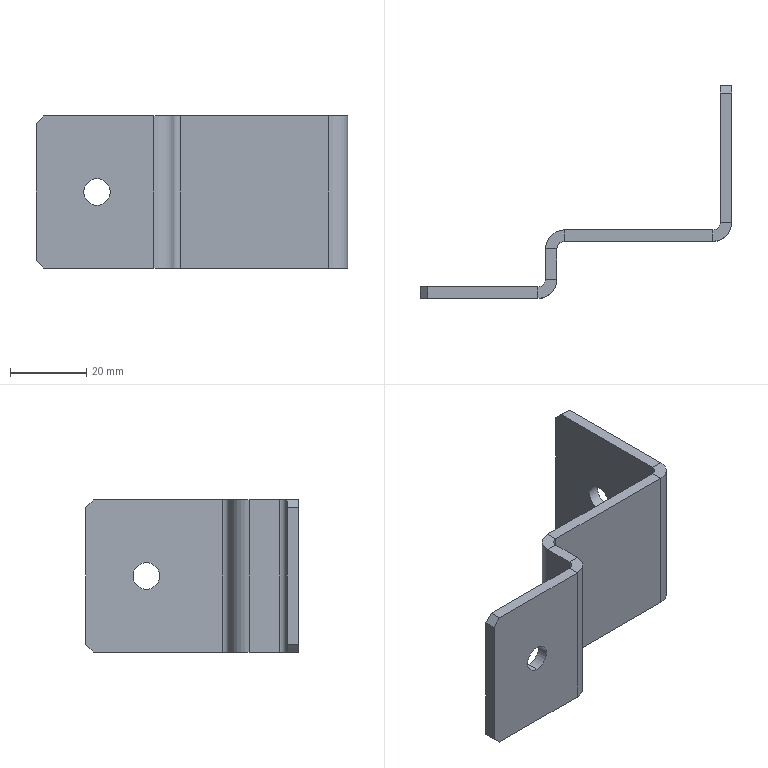Part | NX | features BREP 1 | 1 solid | 38 faces | box 82 x 56 x 40 mm | volume 15404 mm3 | plane 28 | cylinder 10 | commonest cylinder face diameters 7 x4 4 x3 10 x3
STEP:
#1=CARTESIAN_POINT('',(-34.,0.,20.));
#2=VERTEX_POINT('',#1);
#3=CARTESIAN_POINT('',(-36.,0.,18.));
#4=VERTEX_POINT('',#3);
#5=CARTESIAN_POINT('',(-36.,0.,18.));
#6=DIRECTION('',(-0.7071,0.,-0.7071));
#7=VECTOR('',#6,1000.);
#8=LINE('',#5,#7);
#9=EDGE_CURVE('',#2,#4,#8,.T.);
#10=ORIENTED_EDGE('',*,*,#9,.F.);
#11=CARTESIAN_POINT('',(-34.,3.,20.));
#12=VERTEX_POINT('',#11);
#13=CARTESIAN_POINT('',(-34.,5.,20.));
#14=DIRECTION('',(0.,-1.,0.));
#15=VECTOR('',#14,1000.);
#16=LINE('',#13,#15);
#17=EDGE_CURVE('',#12,#2,#16,.T.);
#18=ORIENTED_EDGE('',*,*,#17,.F.);
#19=CARTESIAN_POINT('',(-36.,3.,18.));
#20=VERTEX_POINT('',#19);
#21=CARTESIAN_POINT('',(-35.,3.,19.));
#22=DIRECTION('',(0.7071,0.,0.7071));
#23=VECTOR('',#22,1000.);
#24=LINE('',#21,#23);
#25=EDGE_CURVE('',#20,#12,#24,.T.);
#26=ORIENTED_EDGE('',*,*,#25,.F.);
#27=CARTESIAN_POINT('',(-36.,0.,18.));
#28=DIRECTION('',(0.,1.,0.));
#29=VECTOR('',#28,1000.);
#30=LINE('',#27,#29);
#31=EDGE_CURVE('',#4,#20,#30,.T.);
#32=ORIENTED_EDGE('',*,*,#31,.F.);
#33=EDGE_LOOP('',(#10,#18,#26,#32));
#34=FACE_BOUND('',#33,.T.);
#35=CARTESIAN_POINT('',(-36.,0.,18.));
#36=DIRECTION('',(0.7071,0.,-0.7071));
#37=DIRECTION('',(0.,1.,0.));
#38=AXIS2_PLACEMENT_3D('',#35,#36,#37);
#39=PLANE('',#38);
#40=ADVANCED_FACE('',(#34),#39,.F.);
#41=CARTESIAN_POINT('',(-36.,0.,-18.));
#42=VERTEX_POINT('',#41);
#43=CARTESIAN_POINT('',(-34.,0.,-20.));
#44=VERTEX_POINT('',#43);
#45=CARTESIAN_POINT('',(-34.,0.,-20.));
#46=DIRECTION('',(0.7071,0.,-0.7071));
#47=VECTOR('',#46,1000.);
#48=LINE('',#45,#47);
#49=EDGE_CURVE('',#42,#44,#48,.T.);
#50=ORIENTED_EDGE('',*,*,#49,.F.);
#51=CARTESIAN_POINT('',(-36.,3.,-18.));
#52=VERTEX_POINT('',#51);
#53=CARTESIAN_POINT('',(-36.,0.,-18.));
#54=DIRECTION('',(0.,-1.,0.));
#55=VECTOR('',#54,1000.);
#56=LINE('',#53,#55);
#57=EDGE_CURVE('',#52,#42,#56,.T.);
#58=ORIENTED_EDGE('',*,*,#57,.F.);
#59=CARTESIAN_POINT('',(-34.,3.,-20.));
#60=VERTEX_POINT('',#59);
#61=CARTESIAN_POINT('',(-55.,3.,1.));
#62=DIRECTION('',(-0.7071,0.,0.7071));
#63=VECTOR('',#62,1000.);
#64=LINE('',#61,#63);
#65=EDGE_CURVE('',#60,#52,#64,.T.);
#66=ORIENTED_EDGE('',*,*,#65,.F.);
#67=CARTESIAN_POINT('',(-34.,3.,-20.));
#68=DIRECTION('',(0.,1.,0.));
#69=VECTOR('',#68,1000.);
#70=LINE('',#67,#69);
#71=EDGE_CURVE('',#44,#60,#70,.T.);
#72=ORIENTED_EDGE('',*,*,#71,.F.);
#73=EDGE_LOOP('',(#50,#58,#66,#72));
#74=FACE_BOUND('',#73,.T.);
#75=CARTESIAN_POINT('',(-34.,20.,-20.));
#76=DIRECTION('',(-0.7071,0.,-0.7071));
#77=DIRECTION('',(0.,-1.,0.));
#78=AXIS2_PLACEMENT_3D('',#75,#76,#77);
#79=PLANE('',#78);
#80=ADVANCED_FACE('',(#74),#79,.T.);
#81=CARTESIAN_POINT('',(43.,54.,20.));
#82=VERTEX_POINT('',#81);
#83=CARTESIAN_POINT('',(43.,56.,18.));
#84=VERTEX_POINT('',#83);
#85=CARTESIAN_POINT('',(43.,34.5,39.5));
#86=DIRECTION('',(0.,0.7071,-0.7071));
#87=VECTOR('',#86,1000.);
#88=LINE('',#85,#87);
#89=EDGE_CURVE('',#82,#84,#88,.T.);
#90=ORIENTED_EDGE('',*,*,#89,.F.);
#91=CARTESIAN_POINT('',(46.,54.,20.));
#92=VERTEX_POINT('',#91);
#93=CARTESIAN_POINT('',(41.,54.,20.));
#94=DIRECTION('',(-1.,0.,0.));
#95=VECTOR('',#94,1000.);
#96=LINE('',#93,#95);
#97=EDGE_CURVE('',#92,#82,#96,.T.);
#98=ORIENTED_EDGE('',*,*,#97,.F.);
#99=CARTESIAN_POINT('',(46.,56.,18.));
#100=VERTEX_POINT('',#99);
#101=CARTESIAN_POINT('',(46.,56.,18.));
#102=DIRECTION('',(0.,-0.7071,0.7071));
#103=VECTOR('',#102,1000.);
#104=LINE('',#101,#103);
#105=EDGE_CURVE('',#100,#92,#104,.T.);
#106=ORIENTED_EDGE('',*,*,#105,.F.);
#107=CARTESIAN_POINT('',(43.,56.,18.));
#108=DIRECTION('',(1.,0.,0.));
#109=VECTOR('',#108,1000.);
#110=LINE('',#107,#109);
#111=EDGE_CURVE('',#84,#100,#110,.T.);
#112=ORIENTED_EDGE('',*,*,#111,.F.);
#113=EDGE_LOOP('',(#90,#98,#106,#112));
#114=FACE_BOUND('',#113,.T.);
#115=CARTESIAN_POINT('',(43.,56.,18.));
#116=DIRECTION('',(0.,-0.7071,-0.7071));
#117=DIRECTION('',(1.,0.,0.));
#118=AXIS2_PLACEMENT_3D('',#115,#116,#117);
#119=PLANE('',#118);
#120=ADVANCED_FACE('',(#114),#119,.F.);
#121=CARTESIAN_POINT('',(43.,56.,-18.));
#122=VERTEX_POINT('',#121);
#123=CARTESIAN_POINT('',(43.,54.,-20.));
#124=VERTEX_POINT('',#123);
#125=CARTESIAN_POINT('',(43.,54.5,-19.5));
#126=DIRECTION('',(0.,-0.7071,-0.7071));
#127=VECTOR('',#126,1000.);
#128=LINE('',#125,#127);
#129=EDGE_CURVE('',#122,#124,#128,.T.);
#130=ORIENTED_EDGE('',*,*,#129,.F.);
#131=CARTESIAN_POINT('',(46.,56.,-18.));
#132=VERTEX_POINT('',#131);
#133=CARTESIAN_POINT('',(43.,56.,-18.));
#134=DIRECTION('',(-1.,0.,0.));
#135=VECTOR('',#134,1000.);
#136=LINE('',#133,#135);
#137=EDGE_CURVE('',#132,#122,#136,.T.);
#138=ORIENTED_EDGE('',*,*,#137,.F.);
#139=CARTESIAN_POINT('',(46.,54.,-20.));
#140=VERTEX_POINT('',#139);
#141=CARTESIAN_POINT('',(46.,54.,-20.));
#142=DIRECTION('',(0.,0.7071,0.7071));
#143=VECTOR('',#142,1000.);
#144=LINE('',#141,#143);
#145=EDGE_CURVE('',#140,#132,#144,.T.);
#146=ORIENTED_EDGE('',*,*,#145,.F.);
#147=CARTESIAN_POINT('',(41.,54.,-20.));
#148=DIRECTION('',(1.,0.,0.));
#149=VECTOR('',#148,1000.);
#150=LINE('',#147,#149);
#151=EDGE_CURVE('',#124,#140,#150,.T.);
#152=ORIENTED_EDGE('',*,*,#151,.F.);
#153=EDGE_LOOP('',(#130,#138,#146,#152));
#154=FACE_BOUND('',#153,.T.);
#155=CARTESIAN_POINT('',(41.,54.,-20.));
#156=DIRECTION('',(0.,-0.7071,0.7071));
#157=DIRECTION('',(1.,0.,0.));
#158=AXIS2_PLACEMENT_3D('',#155,#156,#157);
#159=PLANE('',#158);
#160=ADVANCED_FACE('',(#154),#159,.F.);
#161=CARTESIAN_POINT('',(43.,40.,-3.5));
#162=VERTEX_POINT('',#161);
#163=CARTESIAN_POINT('',(46.,40.,-3.5));
#164=VERTEX_POINT('',#163);
#165=CARTESIAN_POINT('',(43.,40.,-3.5));
#166=DIRECTION('',(-1.,0.,0.));
#167=VECTOR('',#166,1000.);
#168=LINE('',#165,#167);
#169=EDGE_CURVE('',#162,#164,#168,.F.);
#170=ORIENTED_EDGE('',*,*,#169,.T.);
#171=CARTESIAN_POINT('',(46.,40.,3.5));
#172=VERTEX_POINT('',#171);
#173=CARTESIAN_POINT('',(46.,40.,0.));
#174=DIRECTION('',(-1.,0.,0.));
#175=DIRECTION('',(0.,0.,1.));
#176=AXIS2_PLACEMENT_3D('',#173,#174,#175);
#177=CIRCLE('',#176,3.5);
#178=EDGE_CURVE('',#172,#164,#177,.T.);
#179=ORIENTED_EDGE('',*,*,#178,.F.);
#180=CARTESIAN_POINT('',(43.,40.,3.5));
#181=VERTEX_POINT('',#180);
#182=CARTESIAN_POINT('',(43.,40.,3.5));
#183=DIRECTION('',(-1.,0.,0.));
#184=VECTOR('',#183,1000.);
#185=LINE('',#182,#184);
#186=EDGE_CURVE('',#181,#172,#185,.F.);
#187=ORIENTED_EDGE('',*,*,#186,.F.);
#188=CARTESIAN_POINT('',(43.,40.,0.));
#189=DIRECTION('',(-1.,0.,0.));
#190=DIRECTION('',(0.,0.,1.));
#191=AXIS2_PLACEMENT_3D('',#188,#189,#190);
#192=CIRCLE('',#191,3.5);
#193=EDGE_CURVE('',#181,#162,#192,.T.);
#194=ORIENTED_EDGE('',*,*,#193,.T.);
#195=EDGE_LOOP('',(#170,#179,#187,#194));
#196=FACE_BOUND('',#195,.T.);
#197=CARTESIAN_POINT('',(43.,40.,0.));
#198=DIRECTION('',(-1.,0.,0.));
#199=DIRECTION('',(0.,0.,1.));
#200=AXIS2_PLACEMENT_3D('',#197,#198,#199);
#201=CYLINDRICAL_SURFACE('',#200,3.5);
#202=ADVANCED_FACE('',(#196),#201,.F.);
#203=CARTESIAN_POINT('',(-20.,3.,-3.5));
#204=VERTEX_POINT('',#203);
#205=CARTESIAN_POINT('',(-20.,0.,-3.5));
#206=VERTEX_POINT('',#205);
#207=CARTESIAN_POINT('',(-20.,3.,-3.5));
#208=DIRECTION('',(0.,1.,0.));
#209=VECTOR('',#208,1000.);
#210=LINE('',#207,#209);
#211=EDGE_CURVE('',#204,#206,#210,.F.);
#212=ORIENTED_EDGE('',*,*,#211,.T.);
#213=CARTESIAN_POINT('',(-20.,0.,3.5));
#214=VERTEX_POINT('',#213);
#215=CARTESIAN_POINT('',(-20.,0.,0.));
#216=DIRECTION('',(0.,1.,0.));
#217=DIRECTION('',(0.,0.,1.));
#218=AXIS2_PLACEMENT_3D('',#215,#216,#217);
#219=CIRCLE('',#218,3.5);
#220=EDGE_CURVE('',#214,#206,#219,.T.);
#221=ORIENTED_EDGE('',*,*,#220,.F.);
#222=CARTESIAN_POINT('',(-20.,3.,3.5));
#223=VERTEX_POINT('',#222);
#224=CARTESIAN_POINT('',(-20.,3.,3.5));
#225=DIRECTION('',(0.,1.,0.));
#226=VECTOR('',#225,1000.);
#227=LINE('',#224,#226);
#228=EDGE_CURVE('',#223,#214,#227,.F.);
#229=ORIENTED_EDGE('',*,*,#228,.F.);
#230=CARTESIAN_POINT('',(-20.,3.,0.));
#231=DIRECTION('',(0.,1.,0.));
#232=DIRECTION('',(0.,0.,1.));
#233=AXIS2_PLACEMENT_3D('',#230,#231,#232);
#234=CIRCLE('',#233,3.5);
#235=EDGE_CURVE('',#223,#204,#234,.T.);
#236=ORIENTED_EDGE('',*,*,#235,.T.);
#237=EDGE_LOOP('',(#212,#221,#229,#236));
#238=FACE_BOUND('',#237,.T.);
#239=CARTESIAN_POINT('',(-20.,3.,0.));
#240=DIRECTION('',(0.,1.,0.));
#241=DIRECTION('',(0.,0.,1.));
#242=AXIS2_PLACEMENT_3D('',#239,#240,#241);
#243=CYLINDRICAL_SURFACE('',#242,3.5);
#244=ADVANCED_FACE('',(#238),#243,.F.);
#245=CARTESIAN_POINT('',(-5.,0.,-20.));
#246=VERTEX_POINT('',#245);
#247=CARTESIAN_POINT('',(-36.,0.,-20.));
#248=DIRECTION('',(1.,0.,0.));
#249=VECTOR('',#248,1000.);
#250=LINE('',#247,#249);
#251=EDGE_CURVE('',#44,#246,#250,.T.);
#252=ORIENTED_EDGE('',*,*,#251,.F.);
#253=ORIENTED_EDGE('',*,*,#71,.T.);
#254=CARTESIAN_POINT('',(-5.,3.,-20.));
#255=VERTEX_POINT('',#254);
#256=CARTESIAN_POINT('',(-36.,3.,-20.));
#257=DIRECTION('',(1.,0.,0.));
#258=VECTOR('',#257,1000.);
#259=LINE('',#256,#258);
#260=EDGE_CURVE('',#60,#255,#259,.T.);
#261=ORIENTED_EDGE('',*,*,#260,.T.);
#262=CARTESIAN_POINT('',(-5.,3.,-20.));
#263=DIRECTION('',(0.,-1.,0.));
#264=VECTOR('',#263,1000.);
#265=LINE('',#262,#264);
#266=EDGE_CURVE('',#255,#246,#265,.T.);
#267=ORIENTED_EDGE('',*,*,#266,.T.);
#268=EDGE_LOOP('',(#252,#253,#261,#267));
#269=FACE_BOUND('',#268,.T.);
#270=CARTESIAN_POINT('',(41.,20.,-20.));
#271=DIRECTION('',(0.,0.,1.));
#272=DIRECTION('',(1.,0.,0.));
#273=AXIS2_PLACEMENT_3D('',#270,#271,#272);
#274=PLANE('',#273);
#275=ADVANCED_FACE('',(#269),#274,.F.);
#276=CARTESIAN_POINT('',(46.,20.,20.));
#277=VERTEX_POINT('',#276);
#278=CARTESIAN_POINT('',(46.,15.,20.));
#279=DIRECTION('',(0.,1.,0.));
#280=VECTOR('',#279,1000.);
#281=LINE('',#278,#280);
#282=EDGE_CURVE('',#277,#92,#281,.T.);
#283=ORIENTED_EDGE('',*,*,#282,.T.);
#284=ORIENTED_EDGE('',*,*,#97,.T.);
#285=CARTESIAN_POINT('',(43.,20.,20.));
#286=VERTEX_POINT('',#285);
#287=CARTESIAN_POINT('',(43.,15.,20.));
#288=DIRECTION('',(0.,1.,0.));
#289=VECTOR('',#288,1000.);
#290=LINE('',#287,#289);
#291=EDGE_CURVE('',#286,#82,#290,.T.);
#292=ORIENTED_EDGE('',*,*,#291,.F.);
#293=CARTESIAN_POINT('',(43.,20.,20.));
#294=DIRECTION('',(1.,0.,0.));
#295=VECTOR('',#294,1000.);
#296=LINE('',#293,#295);
#297=EDGE_CURVE('',#286,#277,#296,.T.);
#298=ORIENTED_EDGE('',*,*,#297,.T.);
#299=EDGE_LOOP('',(#283,#284,#292,#298));
#300=FACE_BOUND('',#299,.T.);
#301=CARTESIAN_POINT('',(41.,20.,20.));
#302=DIRECTION('',(0.,0.,1.));
#303=DIRECTION('',(1.,0.,0.));
#304=AXIS2_PLACEMENT_3D('',#301,#302,#303);
#305=PLANE('',#304);
#306=ADVANCED_FACE('',(#300),#305,.T.);
#307=CARTESIAN_POINT('',(41.,15.,-20.));
#308=VERTEX_POINT('',#307);
#309=CARTESIAN_POINT('',(46.,20.,-20.));
#310=VERTEX_POINT('',#309);
#311=CARTESIAN_POINT('',(41.,20.,-20.));
#312=DIRECTION('',(0.,0.,1.));
#313=DIRECTION('',(-1.,0.,0.));
#314=AXIS2_PLACEMENT_3D('',#311,#312,#313);
#315=CIRCLE('',#314,5.);
#316=EDGE_CURVE('',#308,#310,#315,.T.);
#317=ORIENTED_EDGE('',*,*,#316,.T.);
#318=CARTESIAN_POINT('',(46.,20.,20.));
#319=DIRECTION('',(0.,0.,-1.));
#320=VECTOR('',#319,1000.);
#321=LINE('',#318,#320);
#322=EDGE_CURVE('',#277,#310,#321,.T.);
#323=ORIENTED_EDGE('',*,*,#322,.F.);
#324=CARTESIAN_POINT('',(41.,15.,20.));
#325=VERTEX_POINT('',#324);
#326=CARTESIAN_POINT('',(41.,20.,20.));
#327=DIRECTION('',(0.,0.,1.));
#328=DIRECTION('',(-1.,0.,0.));
#329=AXIS2_PLACEMENT_3D('',#326,#327,#328);
#330=CIRCLE('',#329,5.);
#331=EDGE_CURVE('',#325,#277,#330,.T.);
#332=ORIENTED_EDGE('',*,*,#331,.F.);
#333=CARTESIAN_POINT('',(41.,15.,20.));
#334=DIRECTION('',(0.,0.,-1.));
#335=VECTOR('',#334,1000.);
#336=LINE('',#333,#335);
#337=EDGE_CURVE('',#325,#308,#336,.T.);
#338=ORIENTED_EDGE('',*,*,#337,.T.);
#339=EDGE_LOOP('',(#317,#323,#332,#338));
#340=FACE_BOUND('',#339,.T.);
#341=CARTESIAN_POINT('',(41.,20.,20.));
#342=DIRECTION('',(0.,0.,-1.));
#343=DIRECTION('',(-1.,0.,0.));
#344=AXIS2_PLACEMENT_3D('',#341,#342,#343);
#345=CYLINDRICAL_SURFACE('',#344,5.);
#346=ADVANCED_FACE('',(#340),#345,.T.);
#347=CARTESIAN_POINT('',(2.,15.,-20.));
#348=VERTEX_POINT('',#347);
#349=CARTESIAN_POINT('',(0.,15.,-20.));
#350=DIRECTION('',(1.,0.,0.));
#351=VECTOR('',#350,1000.);
#352=LINE('',#349,#351);
#353=EDGE_CURVE('',#348,#308,#352,.T.);
#354=ORIENTED_EDGE('',*,*,#353,.T.);
#355=ORIENTED_EDGE('',*,*,#337,.F.);
#356=CARTESIAN_POINT('',(2.,15.,20.));
#357=VERTEX_POINT('',#356);
#358=CARTESIAN_POINT('',(0.,15.,20.));
#359=DIRECTION('',(1.,0.,0.));
#360=VECTOR('',#359,1000.);
#361=LINE('',#358,#360);
#362=EDGE_CURVE('',#357,#325,#361,.T.);
#363=ORIENTED_EDGE('',*,*,#362,.F.);
#364=CARTESIAN_POINT('',(2.,15.,20.));
#365=DIRECTION('',(0.,0.,-1.));
#366=VECTOR('',#365,1000.);
#367=LINE('',#364,#366);
#368=EDGE_CURVE('',#357,#348,#367,.T.);
#369=ORIENTED_EDGE('',*,*,#368,.T.);
#370=EDGE_LOOP('',(#354,#355,#363,#369));
#371=FACE_BOUND('',#370,.T.);
#372=CARTESIAN_POINT('',(0.,15.,20.));
#373=DIRECTION('',(0.,1.,0.));
#374=DIRECTION('',(0.,0.,1.));
#375=AXIS2_PLACEMENT_3D('',#372,#373,#374);
#376=PLANE('',#375);
#377=ADVANCED_FACE('',(#371),#376,.F.);
#378=CARTESIAN_POINT('',(0.,13.,-20.));
#379=VERTEX_POINT('',#378);
#380=CARTESIAN_POINT('',(2.,13.,-20.));
#381=DIRECTION('',(0.,0.,-1.));
#382=DIRECTION('',(1.,0.,0.));
#383=AXIS2_PLACEMENT_3D('',#380,#381,#382);
#384=CIRCLE('',#383,2.);
#385=EDGE_CURVE('',#379,#348,#384,.T.);
#386=ORIENTED_EDGE('',*,*,#385,.T.);
#387=ORIENTED_EDGE('',*,*,#368,.F.);
#388=CARTESIAN_POINT('',(0.,13.,20.));
#389=VERTEX_POINT('',#388);
#390=CARTESIAN_POINT('',(2.,13.,20.));
#391=DIRECTION('',(0.,0.,-1.));
#392=DIRECTION('',(1.,0.,0.));
#393=AXIS2_PLACEMENT_3D('',#390,#391,#392);
#394=CIRCLE('',#393,2.);
#395=EDGE_CURVE('',#389,#357,#394,.T.);
#396=ORIENTED_EDGE('',*,*,#395,.F.);
#397=CARTESIAN_POINT('',(0.,13.,20.));
#398=DIRECTION('',(0.,0.,-1.));
#399=VECTOR('',#398,1000.);
#400=LINE('',#397,#399);
#401=EDGE_CURVE('',#389,#379,#400,.T.);
#402=ORIENTED_EDGE('',*,*,#401,.T.);
#403=EDGE_LOOP('',(#386,#387,#396,#402));
#404=FACE_BOUND('',#403,.T.);
#405=CARTESIAN_POINT('',(2.,13.,20.));
#406=DIRECTION('',(0.,0.,-1.));
#407=DIRECTION('',(-1.,0.,0.));
#408=AXIS2_PLACEMENT_3D('',#405,#406,#407);
#409=CYLINDRICAL_SURFACE('',#408,2.);
#410=ADVANCED_FACE('',(#404),#409,.F.);
#411=CARTESIAN_POINT('',(0.,5.,-20.));
#412=VERTEX_POINT('',#411);
#413=CARTESIAN_POINT('',(0.,0.,-20.));
#414=DIRECTION('',(0.,1.,0.));
#415=VECTOR('',#414,1000.);
#416=LINE('',#413,#415);
#417=EDGE_CURVE('',#412,#379,#416,.T.);
#418=ORIENTED_EDGE('',*,*,#417,.T.);
#419=ORIENTED_EDGE('',*,*,#401,.F.);
#420=CARTESIAN_POINT('',(0.,5.,20.));
#421=VERTEX_POINT('',#420);
#422=CARTESIAN_POINT('',(0.,0.,20.));
#423=DIRECTION('',(0.,1.,0.));
#424=VECTOR('',#423,1000.);
#425=LINE('',#422,#424);
#426=EDGE_CURVE('',#421,#389,#425,.T.);
#427=ORIENTED_EDGE('',*,*,#426,.F.);
#428=CARTESIAN_POINT('',(0.,5.,20.));
#429=DIRECTION('',(0.,0.,-1.));
#430=VECTOR('',#429,1000.);
#431=LINE('',#428,#430);
#432=EDGE_CURVE('',#421,#412,#431,.T.);
#433=ORIENTED_EDGE('',*,*,#432,.T.);
#434=EDGE_LOOP('',(#418,#419,#427,#433));
#435=FACE_BOUND('',#434,.T.);
#436=CARTESIAN_POINT('',(0.,0.,20.));
#437=DIRECTION('',(-1.,0.,0.));
#438=DIRECTION('',(0.,0.,1.));
#439=AXIS2_PLACEMENT_3D('',#436,#437,#438);
#440=PLANE('',#439);
#441=ADVANCED_FACE('',(#435),#440,.F.);
#442=CARTESIAN_POINT('',(-5.,5.,-20.));
#443=DIRECTION('',(0.,0.,1.));
#444=DIRECTION('',(-1.,0.,0.));
#445=AXIS2_PLACEMENT_3D('',#442,#443,#444);
#446=CIRCLE('',#445,5.);
#447=EDGE_CURVE('',#246,#412,#446,.T.);
#448=ORIENTED_EDGE('',*,*,#447,.T.);
#449=ORIENTED_EDGE('',*,*,#432,.F.);
#450=CARTESIAN_POINT('',(-5.,0.,20.));
#451=VERTEX_POINT('',#450);
#452=CARTESIAN_POINT('',(-5.,5.,20.));
#453=DIRECTION('',(0.,0.,1.));
#454=DIRECTION('',(-1.,0.,0.));
#455=AXIS2_PLACEMENT_3D('',#452,#453,#454);
#456=CIRCLE('',#455,5.);
#457=EDGE_CURVE('',#451,#421,#456,.T.);
#458=ORIENTED_EDGE('',*,*,#457,.F.);
#459=CARTESIAN_POINT('',(-5.,0.,20.));
#460=DIRECTION('',(0.,0.,-1.));
#461=VECTOR('',#460,1000.);
#462=LINE('',#459,#461);
#463=EDGE_CURVE('',#451,#246,#462,.T.);
#464=ORIENTED_EDGE('',*,*,#463,.T.);
#465=EDGE_LOOP('',(#448,#449,#458,#464));
#466=FACE_BOUND('',#465,.T.);
#467=CARTESIAN_POINT('',(-5.,5.,20.));
#468=DIRECTION('',(0.,0.,-1.));
#469=DIRECTION('',(-1.,0.,0.));
#470=AXIS2_PLACEMENT_3D('',#467,#468,#469);
#471=CYLINDRICAL_SURFACE('',#470,5.);
#472=ADVANCED_FACE('',(#466),#471,.T.);
#473=CARTESIAN_POINT('',(-36.,0.,20.));
#474=DIRECTION('',(0.,0.,-1.));
#475=VECTOR('',#474,1000.);
#476=LINE('',#473,#475);
#477=EDGE_CURVE('',#4,#42,#476,.T.);
#478=ORIENTED_EDGE('',*,*,#477,.T.);
#479=ORIENTED_EDGE('',*,*,#49,.T.);
#480=ORIENTED_EDGE('',*,*,#251,.T.);
#481=ORIENTED_EDGE('',*,*,#463,.F.);
#482=CARTESIAN_POINT('',(-36.,0.,20.));
#483=DIRECTION('',(1.,0.,0.));
#484=VECTOR('',#483,1000.);
#485=LINE('',#482,#484);
#486=EDGE_CURVE('',#2,#451,#485,.T.);
#487=ORIENTED_EDGE('',*,*,#486,.F.);
#488=ORIENTED_EDGE('',*,*,#9,.T.);
#489=EDGE_LOOP('',(#478,#479,#480,#481,#487,#488));
#490=FACE_BOUND('',#489,.T.);
#491=ORIENTED_EDGE('',*,*,#220,.T.);
#492=CARTESIAN_POINT('',(-20.,0.,0.));
#493=DIRECTION('',(0.,1.,0.));
#494=DIRECTION('',(0.,0.,1.));
#495=AXIS2_PLACEMENT_3D('',#492,#493,#494);
#496=CIRCLE('',#495,3.5);
#497=EDGE_CURVE('',#206,#214,#496,.T.);
#498=ORIENTED_EDGE('',*,*,#497,.T.);
#499=EDGE_LOOP('',(#491,#498));
#500=FACE_BOUND('',#499,.T.);
#501=CARTESIAN_POINT('',(-36.,0.,20.));
#502=DIRECTION('',(0.,1.,0.));
#503=DIRECTION('',(0.,0.,1.));
#504=AXIS2_PLACEMENT_3D('',#501,#502,#503);
#505=PLANE('',#504);
#506=ADVANCED_FACE('',(#490,#500),#505,.F.);
#507=CARTESIAN_POINT('',(-36.,3.,20.));
#508=DIRECTION('',(0.,0.,-1.));
#509=VECTOR('',#508,1000.);
#510=LINE('',#507,#509);
#511=EDGE_CURVE('',#20,#52,#510,.T.);
#512=ORIENTED_EDGE('',*,*,#511,.T.);
#513=ORIENTED_EDGE('',*,*,#57,.T.);
#514=ORIENTED_EDGE('',*,*,#477,.F.);
#515=ORIENTED_EDGE('',*,*,#31,.T.);
#516=EDGE_LOOP('',(#512,#513,#514,#515));
#517=FACE_BOUND('',#516,.T.);
#518=CARTESIAN_POINT('',(-36.,0.,20.));
#519=DIRECTION('',(-1.,0.,0.));
#520=DIRECTION('',(0.,0.,1.));
#521=AXIS2_PLACEMENT_3D('',#518,#519,#520);
#522=PLANE('',#521);
#523=ADVANCED_FACE('',(#517),#522,.T.);
#524=ORIENTED_EDGE('',*,*,#260,.F.);
#525=ORIENTED_EDGE('',*,*,#65,.T.);
#526=ORIENTED_EDGE('',*,*,#511,.F.);
#527=ORIENTED_EDGE('',*,*,#25,.T.);
#528=CARTESIAN_POINT('',(-5.,3.,20.));
#529=VERTEX_POINT('',#528);
#530=CARTESIAN_POINT('',(-36.,3.,20.));
#531=DIRECTION('',(1.,0.,0.));
#532=VECTOR('',#531,1000.);
#533=LINE('',#530,#532);
#534=EDGE_CURVE('',#12,#529,#533,.T.);
#535=ORIENTED_EDGE('',*,*,#534,.T.);
#536=CARTESIAN_POINT('',(-5.,3.,20.));
#537=DIRECTION('',(0.,0.,-1.));
#538=VECTOR('',#537,1000.);
#539=LINE('',#536,#538);
#540=EDGE_CURVE('',#529,#255,#539,.T.);
#541=ORIENTED_EDGE('',*,*,#540,.T.);
#542=EDGE_LOOP('',(#524,#525,#526,#527,#535,#541));
#543=FACE_BOUND('',#542,.T.);
#544=ORIENTED_EDGE('',*,*,#235,.F.);
#545=CARTESIAN_POINT('',(-20.,3.,0.));
#546=DIRECTION('',(0.,1.,0.));
#547=DIRECTION('',(0.,0.,1.));
#548=AXIS2_PLACEMENT_3D('',#545,#546,#547);
#549=CIRCLE('',#548,3.5);
#550=EDGE_CURVE('',#204,#223,#549,.T.);
#551=ORIENTED_EDGE('',*,*,#550,.F.);
#552=EDGE_LOOP('',(#544,#551));
#553=FACE_BOUND('',#552,.T.);
#554=CARTESIAN_POINT('',(-36.,3.,20.));
#555=DIRECTION('',(0.,1.,0.));
#556=DIRECTION('',(0.,0.,1.));
#557=AXIS2_PLACEMENT_3D('',#554,#555,#556);
#558=PLANE('',#557);
#559=ADVANCED_FACE('',(#543,#553),#558,.T.);
#560=CARTESIAN_POINT('',(-3.,5.,-20.));
#561=VERTEX_POINT('',#560);
#562=CARTESIAN_POINT('',(-5.,5.,-20.));
#563=DIRECTION('',(0.,0.,1.));
#564=DIRECTION('',(1.,0.,0.));
#565=AXIS2_PLACEMENT_3D('',#562,#563,#564);
#566=CIRCLE('',#565,2.);
#567=EDGE_CURVE('',#255,#561,#566,.T.);
#568=ORIENTED_EDGE('',*,*,#567,.F.);
#569=ORIENTED_EDGE('',*,*,#540,.F.);
#570=CARTESIAN_POINT('',(-3.,5.,20.));
#571=VERTEX_POINT('',#570);
#572=CARTESIAN_POINT('',(-5.,5.,20.));
#573=DIRECTION('',(0.,0.,1.));
#574=DIRECTION('',(1.,0.,0.));
#575=AXIS2_PLACEMENT_3D('',#572,#573,#574);
#576=CIRCLE('',#575,2.);
#577=EDGE_CURVE('',#529,#571,#576,.T.);
#578=ORIENTED_EDGE('',*,*,#577,.T.);
#579=CARTESIAN_POINT('',(-3.,5.,20.));
#580=DIRECTION('',(0.,0.,-1.));
#581=VECTOR('',#580,1000.);
#582=LINE('',#579,#581);
#583=EDGE_CURVE('',#571,#561,#582,.T.);
#584=ORIENTED_EDGE('',*,*,#583,.T.);
#585=EDGE_LOOP('',(#568,#569,#578,#584));
#586=FACE_BOUND('',#585,.T.);
#587=CARTESIAN_POINT('',(-5.,5.,20.));
#588=DIRECTION('',(0.,0.,-1.));
#589=DIRECTION('',(-1.,0.,0.));
#590=AXIS2_PLACEMENT_3D('',#587,#588,#589);
#591=CYLINDRICAL_SURFACE('',#590,2.);
#592=ADVANCED_FACE('',(#586),#591,.F.);
#593=CARTESIAN_POINT('',(-3.,13.,-20.));
#594=VERTEX_POINT('',#593);
#595=CARTESIAN_POINT('',(-3.,0.,-20.));
#596=DIRECTION('',(0.,1.,0.));
#597=VECTOR('',#596,1000.);
#598=LINE('',#595,#597);
#599=EDGE_CURVE('',#561,#594,#598,.T.);
#600=ORIENTED_EDGE('',*,*,#599,.F.);
#601=ORIENTED_EDGE('',*,*,#583,.F.);
#602=CARTESIAN_POINT('',(-3.,13.,20.));
#603=VERTEX_POINT('',#602);
#604=CARTESIAN_POINT('',(-3.,0.,20.));
#605=DIRECTION('',(0.,1.,0.));
#606=VECTOR('',#605,1000.);
#607=LINE('',#604,#606);
#608=EDGE_CURVE('',#571,#603,#607,.T.);
#609=ORIENTED_EDGE('',*,*,#608,.T.);
#610=CARTESIAN_POINT('',(-3.,13.,20.));
#611=DIRECTION('',(0.,0.,-1.));
#612=VECTOR('',#611,1000.);
#613=LINE('',#610,#612);
#614=EDGE_CURVE('',#603,#594,#613,.T.);
#615=ORIENTED_EDGE('',*,*,#614,.T.);
#616=EDGE_LOOP('',(#600,#601,#609,#615));
#617=FACE_BOUND('',#616,.T.);
#618=CARTESIAN_POINT('',(-3.,0.,20.));
#619=DIRECTION('',(-1.,0.,0.));
#620=DIRECTION('',(0.,0.,1.));
#621=AXIS2_PLACEMENT_3D('',#618,#619,#620);
#622=PLANE('',#621);
#623=ADVANCED_FACE('',(#617),#622,.T.);
#624=CARTESIAN_POINT('',(2.,18.,-20.));
#625=VERTEX_POINT('',#624);
#626=CARTESIAN_POINT('',(2.,13.,-20.));
#627=DIRECTION('',(0.,0.,-1.));
#628=DIRECTION('',(1.,0.,0.));
#629=AXIS2_PLACEMENT_3D('',#626,#627,#628);
#630=CIRCLE('',#629,5.);
#631=EDGE_CURVE('',#594,#625,#630,.T.);
#632=ORIENTED_EDGE('',*,*,#631,.F.);
#633=ORIENTED_EDGE('',*,*,#614,.F.);
#634=CARTESIAN_POINT('',(2.,18.,20.));
#635=VERTEX_POINT('',#634);
#636=CARTESIAN_POINT('',(2.,13.,20.));
#637=DIRECTION('',(0.,0.,-1.));
#638=DIRECTION('',(1.,0.,0.));
#639=AXIS2_PLACEMENT_3D('',#636,#637,#638);
#640=CIRCLE('',#639,5.);
#641=EDGE_CURVE('',#603,#635,#640,.T.);
#642=ORIENTED_EDGE('',*,*,#641,.T.);
#643=CARTESIAN_POINT('',(2.,18.,20.));
#644=DIRECTION('',(0.,0.,-1.));
#645=VECTOR('',#644,1000.);
#646=LINE('',#643,#645);
#647=EDGE_CURVE('',#635,#625,#646,.T.);
#648=ORIENTED_EDGE('',*,*,#647,.T.);
#649=EDGE_LOOP('',(#632,#633,#642,#648));
#650=FACE_BOUND('',#649,.T.);
#651=CARTESIAN_POINT('',(2.,13.,20.));
#652=DIRECTION('',(0.,0.,-1.));
#653=DIRECTION('',(-1.,0.,0.));
#654=AXIS2_PLACEMENT_3D('',#651,#652,#653);
#655=CYLINDRICAL_SURFACE('',#654,5.);
#656=ADVANCED_FACE('',(#650),#655,.T.);
#657=CARTESIAN_POINT('',(41.,18.,-20.));
#658=VERTEX_POINT('',#657);
#659=CARTESIAN_POINT('',(0.,18.,-20.));
#660=DIRECTION('',(1.,0.,0.));
#661=VECTOR('',#660,1000.);
#662=LINE('',#659,#661);
#663=EDGE_CURVE('',#625,#658,#662,.T.);
#664=ORIENTED_EDGE('',*,*,#663,.F.);
#665=ORIENTED_EDGE('',*,*,#647,.F.);
#666=CARTESIAN_POINT('',(41.,18.,20.));
#667=VERTEX_POINT('',#666);
#668=CARTESIAN_POINT('',(0.,18.,20.));
#669=DIRECTION('',(1.,0.,0.));
#670=VECTOR('',#669,1000.);
#671=LINE('',#668,#670);
#672=EDGE_CURVE('',#635,#667,#671,.T.);
#673=ORIENTED_EDGE('',*,*,#672,.T.);
#674=CARTESIAN_POINT('',(41.,18.,20.));
#675=DIRECTION('',(0.,0.,-1.));
#676=VECTOR('',#675,1000.);
#677=LINE('',#674,#676);
#678=EDGE_CURVE('',#667,#658,#677,.T.);
#679=ORIENTED_EDGE('',*,*,#678,.T.);
#680=EDGE_LOOP('',(#664,#665,#673,#679));
#681=FACE_BOUND('',#680,.T.);
#682=CARTESIAN_POINT('',(0.,18.,20.));
#683=DIRECTION('',(0.,1.,0.));
#684=DIRECTION('',(0.,0.,1.));
#685=AXIS2_PLACEMENT_3D('',#682,#683,#684);
#686=PLANE('',#685);
#687=ADVANCED_FACE('',(#681),#686,.T.);
#688=CARTESIAN_POINT('',(43.,20.,-20.));
#689=VERTEX_POINT('',#688);
#690=CARTESIAN_POINT('',(41.,20.,-20.));
#691=DIRECTION('',(0.,0.,1.));
#692=DIRECTION('',(1.,0.,0.));
#693=AXIS2_PLACEMENT_3D('',#690,#691,#692);
#694=CIRCLE('',#693,2.);
#695=EDGE_CURVE('',#658,#689,#694,.T.);
#696=ORIENTED_EDGE('',*,*,#695,.F.);
#697=ORIENTED_EDGE('',*,*,#678,.F.);
#698=CARTESIAN_POINT('',(41.,20.,20.));
#699=DIRECTION('',(0.,0.,1.));
#700=DIRECTION('',(1.,0.,0.));
#701=AXIS2_PLACEMENT_3D('',#698,#699,#700);
#702=CIRCLE('',#701,2.);
#703=EDGE_CURVE('',#667,#286,#702,.T.);
#704=ORIENTED_EDGE('',*,*,#703,.T.);
#705=CARTESIAN_POINT('',(43.,20.,20.));
#706=DIRECTION('',(0.,0.,-1.));
#707=VECTOR('',#706,1000.);
#708=LINE('',#705,#707);
#709=EDGE_CURVE('',#286,#689,#708,.T.);
#710=ORIENTED_EDGE('',*,*,#709,.T.);
#711=EDGE_LOOP('',(#696,#697,#704,#710));
#712=FACE_BOUND('',#711,.T.);
#713=CARTESIAN_POINT('',(41.,20.,20.));
#714=DIRECTION('',(0.,0.,-1.));
#715=DIRECTION('',(-1.,0.,0.));
#716=AXIS2_PLACEMENT_3D('',#713,#714,#715);
#717=CYLINDRICAL_SURFACE('',#716,2.);
#718=ADVANCED_FACE('',(#712),#717,.F.);
#719=CARTESIAN_POINT('',(43.,56.,20.));
#720=DIRECTION('',(0.,0.,-1.));
#721=VECTOR('',#720,1000.);
#722=LINE('',#719,#721);
#723=EDGE_CURVE('',#84,#122,#722,.T.);
#724=ORIENTED_EDGE('',*,*,#723,.T.);
#725=ORIENTED_EDGE('',*,*,#129,.T.);
#726=CARTESIAN_POINT('',(43.,15.,-20.));
#727=DIRECTION('',(0.,1.,0.));
#728=VECTOR('',#727,1000.);
#729=LINE('',#726,#728);
#730=EDGE_CURVE('',#689,#124,#729,.T.);
#731=ORIENTED_EDGE('',*,*,#730,.F.);
#732=ORIENTED_EDGE('',*,*,#709,.F.);
#733=ORIENTED_EDGE('',*,*,#291,.T.);
#734=ORIENTED_EDGE('',*,*,#89,.T.);
#735=EDGE_LOOP('',(#724,#725,#731,#732,#733,#734));
#736=FACE_BOUND('',#735,.T.);
#737=ORIENTED_EDGE('',*,*,#193,.F.);
#738=CARTESIAN_POINT('',(43.,40.,0.));
#739=DIRECTION('',(-1.,0.,0.));
#740=DIRECTION('',(0.,0.,1.));
#741=AXIS2_PLACEMENT_3D('',#738,#739,#740);
#742=CIRCLE('',#741,3.5);
#743=EDGE_CURVE('',#162,#181,#742,.T.);
#744=ORIENTED_EDGE('',*,*,#743,.F.);
#745=EDGE_LOOP('',(#737,#744));
#746=FACE_BOUND('',#745,.T.);
#747=CARTESIAN_POINT('',(43.,15.,20.));
#748=DIRECTION('',(-1.,0.,0.));
#749=DIRECTION('',(0.,-1.,0.));
#750=AXIS2_PLACEMENT_3D('',#747,#748,#749);
#751=PLANE('',#750);
#752=ADVANCED_FACE('',(#736,#746),#751,.T.);
#753=CARTESIAN_POINT('',(46.,56.,20.));
#754=DIRECTION('',(0.,0.,-1.));
#755=VECTOR('',#754,1000.);
#756=LINE('',#753,#755);
#757=EDGE_CURVE('',#100,#132,#756,.T.);
#758=ORIENTED_EDGE('',*,*,#757,.T.);
#759=ORIENTED_EDGE('',*,*,#137,.T.);
#760=ORIENTED_EDGE('',*,*,#723,.F.);
#761=ORIENTED_EDGE('',*,*,#111,.T.);
#762=EDGE_LOOP('',(#758,#759,#760,#761));
#763=FACE_BOUND('',#762,.T.);
#764=CARTESIAN_POINT('',(43.,56.,20.));
#765=DIRECTION('',(0.,1.,0.));
#766=DIRECTION('',(0.,0.,1.));
#767=AXIS2_PLACEMENT_3D('',#764,#765,#766);
#768=PLANE('',#767);
#769=ADVANCED_FACE('',(#763),#768,.T.);
#770=CARTESIAN_POINT('',(46.,15.,-20.));
#771=DIRECTION('',(0.,1.,0.));
#772=VECTOR('',#771,1000.);
#773=LINE('',#770,#772);
#774=EDGE_CURVE('',#310,#140,#773,.T.);
#775=ORIENTED_EDGE('',*,*,#774,.T.);
#776=ORIENTED_EDGE('',*,*,#145,.T.);
#777=ORIENTED_EDGE('',*,*,#757,.F.);
#778=ORIENTED_EDGE('',*,*,#105,.T.);
#779=ORIENTED_EDGE('',*,*,#282,.F.);
#780=ORIENTED_EDGE('',*,*,#322,.T.);
#781=EDGE_LOOP('',(#775,#776,#777,#778,#779,#780));
#782=FACE_BOUND('',#781,.T.);
#783=ORIENTED_EDGE('',*,*,#178,.T.);
#784=CARTESIAN_POINT('',(46.,40.,0.));
#785=DIRECTION('',(-1.,0.,0.));
#786=DIRECTION('',(0.,0.,1.));
#787=AXIS2_PLACEMENT_3D('',#784,#785,#786);
#788=CIRCLE('',#787,3.5);
#789=EDGE_CURVE('',#164,#172,#788,.T.);
#790=ORIENTED_EDGE('',*,*,#789,.T.);
#791=EDGE_LOOP('',(#783,#790));
#792=FACE_BOUND('',#791,.T.);
#793=CARTESIAN_POINT('',(46.,15.,20.));
#794=DIRECTION('',(-1.,0.,0.));
#795=DIRECTION('',(0.,-1.,0.));
#796=AXIS2_PLACEMENT_3D('',#793,#794,#795);
#797=PLANE('',#796);
#798=ADVANCED_FACE('',(#782,#792),#797,.F.);
#799=ORIENTED_EDGE('',*,*,#730,.T.);
#800=ORIENTED_EDGE('',*,*,#151,.T.);
#801=ORIENTED_EDGE('',*,*,#774,.F.);
#802=CARTESIAN_POINT('',(46.,20.,-20.));
#803=DIRECTION('',(-1.,0.,0.));
#804=VECTOR('',#803,1000.);
#805=LINE('',#802,#804);
#806=EDGE_CURVE('',#310,#689,#805,.T.);
#807=ORIENTED_EDGE('',*,*,#806,.T.);
#808=EDGE_LOOP('',(#799,#800,#801,#807));
#809=FACE_BOUND('',#808,.T.);
#810=CARTESIAN_POINT('',(41.,18.,-20.));
#811=DIRECTION('',(0.,0.,-1.));
#812=DIRECTION('',(-1.,0.,0.));
#813=AXIS2_PLACEMENT_3D('',#810,#811,#812);
#814=PLANE('',#813);
#815=ADVANCED_FACE('',(#809),#814,.T.);
#816=ORIENTED_EDGE('',*,*,#806,.F.);
#817=ORIENTED_EDGE('',*,*,#316,.F.);
#818=CARTESIAN_POINT('',(41.,18.,-20.));
#819=DIRECTION('',(0.,-1.,0.));
#820=VECTOR('',#819,1000.);
#821=LINE('',#818,#820);
#822=EDGE_CURVE('',#658,#308,#821,.T.);
#823=ORIENTED_EDGE('',*,*,#822,.F.);
#824=ORIENTED_EDGE('',*,*,#695,.T.);
#825=EDGE_LOOP('',(#816,#817,#823,#824));
#826=FACE_BOUND('',#825,.T.);
#827=CARTESIAN_POINT('',(46.,20.,-20.));
#828=DIRECTION('',(0.,0.,-1.));
#829=DIRECTION('',(-1.,0.,0.));
#830=AXIS2_PLACEMENT_3D('',#827,#828,#829);
#831=PLANE('',#830);
#832=ADVANCED_FACE('',(#826),#831,.T.);
#833=ORIENTED_EDGE('',*,*,#362,.T.);
#834=CARTESIAN_POINT('',(41.,15.,20.));
#835=DIRECTION('',(0.,1.,0.));
#836=VECTOR('',#835,1000.);
#837=LINE('',#834,#836);
#838=EDGE_CURVE('',#325,#667,#837,.T.);
#839=ORIENTED_EDGE('',*,*,#838,.T.);
#840=ORIENTED_EDGE('',*,*,#672,.F.);
#841=CARTESIAN_POINT('',(2.,18.,20.));
#842=DIRECTION('',(0.,-1.,0.));
#843=VECTOR('',#842,1000.);
#844=LINE('',#841,#843);
#845=EDGE_CURVE('',#635,#357,#844,.T.);
#846=ORIENTED_EDGE('',*,*,#845,.T.);
#847=EDGE_LOOP('',(#833,#839,#840,#846));
#848=FACE_BOUND('',#847,.T.);
#849=CARTESIAN_POINT('',(43.,20.,20.));
#850=DIRECTION('',(0.,0.,1.));
#851=DIRECTION('',(1.,0.,0.));
#852=AXIS2_PLACEMENT_3D('',#849,#850,#851);
#853=PLANE('',#852);
#854=ADVANCED_FACE('',(#848),#853,.T.);
#855=ORIENTED_EDGE('',*,*,#838,.F.);
#856=ORIENTED_EDGE('',*,*,#331,.T.);
#857=ORIENTED_EDGE('',*,*,#297,.F.);
#858=ORIENTED_EDGE('',*,*,#703,.F.);
#859=EDGE_LOOP('',(#855,#856,#857,#858));
#860=FACE_BOUND('',#859,.T.);
#861=CARTESIAN_POINT('',(41.,15.,20.));
#862=DIRECTION('',(0.,0.,1.));
#863=DIRECTION('',(1.,0.,0.));
#864=AXIS2_PLACEMENT_3D('',#861,#862,#863);
#865=PLANE('',#864);
#866=ADVANCED_FACE('',(#860),#865,.T.);
#867=ORIENTED_EDGE('',*,*,#353,.F.);
#868=CARTESIAN_POINT('',(2.,15.,-20.));
#869=DIRECTION('',(0.,1.,0.));
#870=VECTOR('',#869,1000.);
#871=LINE('',#868,#870);
#872=EDGE_CURVE('',#348,#625,#871,.T.);
#873=ORIENTED_EDGE('',*,*,#872,.T.);
#874=ORIENTED_EDGE('',*,*,#663,.T.);
#875=ORIENTED_EDGE('',*,*,#822,.T.);
#876=EDGE_LOOP('',(#867,#873,#874,#875));
#877=FACE_BOUND('',#876,.T.);
#878=CARTESIAN_POINT('',(-3.,13.,-20.));
#879=DIRECTION('',(0.,0.,-1.));
#880=DIRECTION('',(-1.,0.,0.));
#881=AXIS2_PLACEMENT_3D('',#878,#879,#880);
#882=PLANE('',#881);
#883=ADVANCED_FACE('',(#877),#882,.T.);
#884=ORIENTED_EDGE('',*,*,#872,.F.);
#885=ORIENTED_EDGE('',*,*,#385,.F.);
#886=CARTESIAN_POINT('',(-3.,13.,-20.));
#887=DIRECTION('',(1.,0.,0.));
#888=VECTOR('',#887,1000.);
#889=LINE('',#886,#888);
#890=EDGE_CURVE('',#594,#379,#889,.T.);
#891=ORIENTED_EDGE('',*,*,#890,.F.);
#892=ORIENTED_EDGE('',*,*,#631,.T.);
#893=EDGE_LOOP('',(#884,#885,#891,#892));
#894=FACE_BOUND('',#893,.T.);
#895=CARTESIAN_POINT('',(2.,15.,-20.));
#896=DIRECTION('',(0.,0.,-1.));
#897=DIRECTION('',(-1.,0.,0.));
#898=AXIS2_PLACEMENT_3D('',#895,#896,#897);
#899=PLANE('',#898);
#900=ADVANCED_FACE('',(#894),#899,.T.);
#901=ORIENTED_EDGE('',*,*,#426,.T.);
#902=CARTESIAN_POINT('',(0.,13.,20.));
#903=DIRECTION('',(-1.,0.,0.));
#904=VECTOR('',#903,1000.);
#905=LINE('',#902,#904);
#906=EDGE_CURVE('',#389,#603,#905,.T.);
#907=ORIENTED_EDGE('',*,*,#906,.T.);
#908=ORIENTED_EDGE('',*,*,#608,.F.);
#909=CARTESIAN_POINT('',(-3.,5.,20.));
#910=DIRECTION('',(1.,0.,0.));
#911=VECTOR('',#910,1000.);
#912=LINE('',#909,#911);
#913=EDGE_CURVE('',#571,#421,#912,.T.);
#914=ORIENTED_EDGE('',*,*,#913,.T.);
#915=EDGE_LOOP('',(#901,#907,#908,#914));
#916=FACE_BOUND('',#915,.T.);
#917=CARTESIAN_POINT('',(2.,18.,20.));
#918=DIRECTION('',(0.,0.,1.));
#919=DIRECTION('',(1.,0.,0.));
#920=AXIS2_PLACEMENT_3D('',#917,#918,#919);
#921=PLANE('',#920);
#922=ADVANCED_FACE('',(#916),#921,.T.);
#923=ORIENTED_EDGE('',*,*,#906,.F.);
#924=ORIENTED_EDGE('',*,*,#395,.T.);
#925=ORIENTED_EDGE('',*,*,#845,.F.);
#926=ORIENTED_EDGE('',*,*,#641,.F.);
#927=EDGE_LOOP('',(#923,#924,#925,#926));
#928=FACE_BOUND('',#927,.T.);
#929=CARTESIAN_POINT('',(0.,13.,20.));
#930=DIRECTION('',(0.,0.,1.));
#931=DIRECTION('',(1.,0.,0.));
#932=AXIS2_PLACEMENT_3D('',#929,#930,#931);
#933=PLANE('',#932);
#934=ADVANCED_FACE('',(#928),#933,.T.);
#935=ORIENTED_EDGE('',*,*,#417,.F.);
#936=CARTESIAN_POINT('',(0.,5.,-20.));
#937=DIRECTION('',(-1.,0.,0.));
#938=VECTOR('',#937,1000.);
#939=LINE('',#936,#938);
#940=EDGE_CURVE('',#412,#561,#939,.T.);
#941=ORIENTED_EDGE('',*,*,#940,.T.);
#942=ORIENTED_EDGE('',*,*,#599,.T.);
#943=ORIENTED_EDGE('',*,*,#890,.T.);
#944=EDGE_LOOP('',(#935,#941,#942,#943));
#945=FACE_BOUND('',#944,.T.);
#946=CARTESIAN_POINT('',(-5.,3.,-20.));
#947=DIRECTION('',(0.,0.,-1.));
#948=DIRECTION('',(-1.,0.,0.));
#949=AXIS2_PLACEMENT_3D('',#946,#947,#948);
#950=PLANE('',#949);
#951=ADVANCED_FACE('',(#945),#950,.T.);
#952=ORIENTED_EDGE('',*,*,#940,.F.);
#953=ORIENTED_EDGE('',*,*,#447,.F.);
#954=ORIENTED_EDGE('',*,*,#266,.F.);
#955=ORIENTED_EDGE('',*,*,#567,.T.);
#956=EDGE_LOOP('',(#952,#953,#954,#955));
#957=FACE_BOUND('',#956,.T.);
#958=CARTESIAN_POINT('',(0.,5.,-20.));
#959=DIRECTION('',(0.,0.,-1.));
#960=DIRECTION('',(-1.,0.,0.));
#961=AXIS2_PLACEMENT_3D('',#958,#959,#960);
#962=PLANE('',#961);
#963=ADVANCED_FACE('',(#957),#962,.T.);
#964=ORIENTED_EDGE('',*,*,#534,.F.);
#965=ORIENTED_EDGE('',*,*,#17,.T.);
#966=ORIENTED_EDGE('',*,*,#486,.T.);
#967=CARTESIAN_POINT('',(-5.,0.,20.));
#968=DIRECTION('',(0.,1.,0.));
#969=VECTOR('',#968,1000.);
#970=LINE('',#967,#969);
#971=EDGE_CURVE('',#451,#529,#970,.T.);
#972=ORIENTED_EDGE('',*,*,#971,.T.);
#973=EDGE_LOOP('',(#964,#965,#966,#972));
#974=FACE_BOUND('',#973,.T.);
#975=CARTESIAN_POINT('',(-3.,5.,20.));
#976=DIRECTION('',(0.,0.,1.));
#977=DIRECTION('',(1.,0.,0.));
#978=AXIS2_PLACEMENT_3D('',#975,#976,#977);
#979=PLANE('',#978);
#980=ADVANCED_FACE('',(#974),#979,.T.);
#981=ORIENTED_EDGE('',*,*,#971,.F.);
#982=ORIENTED_EDGE('',*,*,#457,.T.);
#983=ORIENTED_EDGE('',*,*,#913,.F.);
#984=ORIENTED_EDGE('',*,*,#577,.F.);
#985=EDGE_LOOP('',(#981,#982,#983,#984));
#986=FACE_BOUND('',#985,.T.);
#987=CARTESIAN_POINT('',(-5.,0.,20.));
#988=DIRECTION('',(0.,0.,1.));
#989=DIRECTION('',(1.,0.,0.));
#990=AXIS2_PLACEMENT_3D('',#987,#988,#989);
#991=PLANE('',#990);
#992=ADVANCED_FACE('',(#986),#991,.T.);
#993=ORIENTED_EDGE('',*,*,#497,.F.);
#994=ORIENTED_EDGE('',*,*,#211,.F.);
#995=ORIENTED_EDGE('',*,*,#550,.T.);
#996=ORIENTED_EDGE('',*,*,#228,.T.);
#997=EDGE_LOOP('',(#993,#994,#995,#996));
#998=FACE_BOUND('',#997,.T.);
#999=CARTESIAN_POINT('',(-20.,3.,0.));
#1000=DIRECTION('',(0.,1.,0.));
#1001=DIRECTION('',(0.,0.,1.));
#1002=AXIS2_PLACEMENT_3D('',#999,#1000,#1001);
#1003=CYLINDRICAL_SURFACE('',#1002,3.5);
#1004=ADVANCED_FACE('',(#998),#1003,.F.);
#1005=ORIENTED_EDGE('',*,*,#789,.F.);
#1006=ORIENTED_EDGE('',*,*,#169,.F.);
#1007=ORIENTED_EDGE('',*,*,#743,.T.);
#1008=ORIENTED_EDGE('',*,*,#186,.T.);
#1009=EDGE_LOOP('',(#1005,#1006,#1007,#1008));
#1010=FACE_BOUND('',#1009,.T.);
#1011=CARTESIAN_POINT('',(43.,40.,0.));
#1012=DIRECTION('',(-1.,0.,0.));
#1013=DIRECTION('',(0.,0.,1.));
#1014=AXIS2_PLACEMENT_3D('',#1011,#1012,#1013);
#1015=CYLINDRICAL_SURFACE('',#1014,3.5);
#1016=ADVANCED_FACE('',(#1010),#1015,.F.);
#1017=CLOSED_SHELL('',(#40,#80,#120,#160,#202,#244,#275,#306,#346,#377,#410,#441,#472,#506,#523,#559,#592,#623,#656,#687,#718,#752,#769,#798,#815,#832,#854,#866,#883,#900,#922,#934,#951,#963,#980,#992,#1004,#1016));
#1018=MANIFOLD_SOLID_BREP('',#1017);
#1019=(LENGTH_UNIT()NAMED_UNIT(*)SI_UNIT(.MILLI.,.METRE.));
#1020=UNCERTAINTY_MEASURE_WITH_UNIT(LENGTH_MEASURE(0.00001),#1019,'','');
#1021=(NAMED_UNIT(*)PLANE_ANGLE_UNIT()SI_UNIT($,.RADIAN.));
#1022=(NAMED_UNIT(*)SI_UNIT($,.STERADIAN.)SOLID_ANGLE_UNIT());
#1023=(GEOMETRIC_REPRESENTATION_CONTEXT(3)GLOBAL_UNCERTAINTY_ASSIGNED_CONTEXT((#1020))GLOBAL_UNIT_ASSIGNED_CONTEXT((#1019,#1021,#1022))REPRESENTATION_CONTEXT('',''));
#1024=ADVANCED_BREP_SHAPE_REPRESENTATION('',(#1018),#1023);